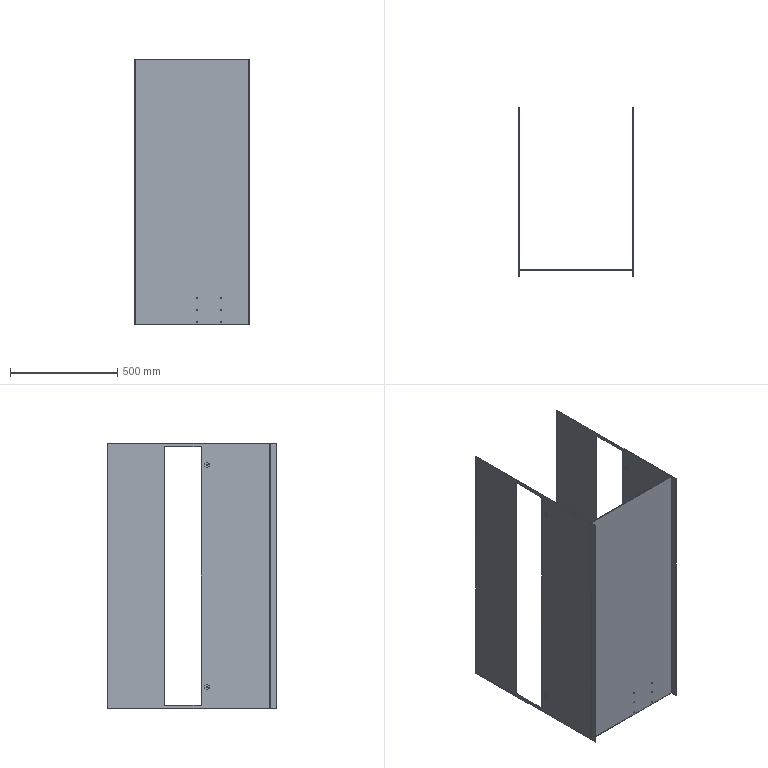Part | SolidWorks | features BaseBody 1 | 1 solid | 90 faces | box 534 x 786.319 x 1236 mm | volume 4372882 mm3 | cylinder 68 | plane 22 | commonest cylinder face diameters 2.021 x48 5.365 x12 3 x8